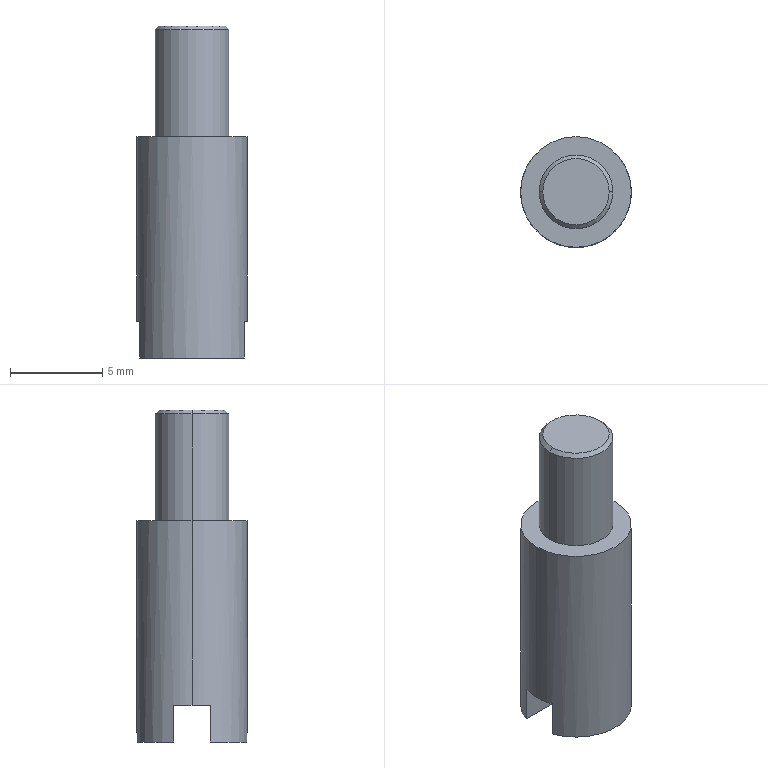Part | NX | features BREP 1 | 1 solid | 13 faces | box 6 x 6 x 18 mm | volume 390.899 mm3 | plane 7 | cylinder 4 | cone 2 | commonest cylinder face diameters 4 x2 6 x2
STEP:
#1=CARTESIAN_POINT('',(-2.828,1.,2.));
#2=VERTEX_POINT('',#1);
#3=CARTESIAN_POINT('',(2.828,1.,2.));
#4=VERTEX_POINT('',#3);
#5=CARTESIAN_POINT('',(3.,1.,2.));
#6=DIRECTION('',(1.,0.,0.));
#7=VECTOR('',#6,1000.);
#8=LINE('',#5,#7);
#9=EDGE_CURVE('',#2,#4,#8,.T.);
#10=ORIENTED_EDGE('',*,*,#9,.F.);
#11=CARTESIAN_POINT('',(-2.828,1.,0.));
#12=VERTEX_POINT('',#11);
#13=CARTESIAN_POINT('',(-2.828,1.,12.));
#14=DIRECTION('',(0.,0.,1.));
#15=VECTOR('',#14,1000.);
#16=LINE('',#13,#15);
#17=EDGE_CURVE('',#12,#2,#16,.T.);
#18=ORIENTED_EDGE('',*,*,#17,.F.);
#19=CARTESIAN_POINT('',(2.828,1.,0.));
#20=VERTEX_POINT('',#19);
#21=CARTESIAN_POINT('',(0.,1.,0.));
#22=DIRECTION('',(-1.,0.,0.));
#23=VECTOR('',#22,1000.);
#24=LINE('',#21,#23);
#25=EDGE_CURVE('',#20,#12,#24,.T.);
#26=ORIENTED_EDGE('',*,*,#25,.F.);
#27=CARTESIAN_POINT('',(2.828,1.,12.));
#28=DIRECTION('',(0.,0.,-1.));
#29=VECTOR('',#28,1000.);
#30=LINE('',#27,#29);
#31=EDGE_CURVE('',#4,#20,#30,.T.);
#32=ORIENTED_EDGE('',*,*,#31,.F.);
#33=EDGE_LOOP('',(#10,#18,#26,#32));
#34=FACE_BOUND('',#33,.T.);
#35=CARTESIAN_POINT('',(3.,1.,2.));
#36=DIRECTION('',(0.,1.,0.));
#37=DIRECTION('',(0.,0.,1.));
#38=AXIS2_PLACEMENT_3D('',#35,#36,#37);
#39=PLANE('',#38);
#40=ADVANCED_FACE('',(#34),#39,.F.);
#41=CARTESIAN_POINT('',(2.828,-1.,2.));
#42=VERTEX_POINT('',#41);
#43=CARTESIAN_POINT('',(-2.828,-1.,2.));
#44=VERTEX_POINT('',#43);
#45=CARTESIAN_POINT('',(3.,-1.,2.));
#46=DIRECTION('',(-1.,0.,0.));
#47=VECTOR('',#46,1000.);
#48=LINE('',#45,#47);
#49=EDGE_CURVE('',#42,#44,#48,.T.);
#50=ORIENTED_EDGE('',*,*,#49,.F.);
#51=CARTESIAN_POINT('',(2.828,-1.,0.));
#52=VERTEX_POINT('',#51);
#53=CARTESIAN_POINT('',(2.828,-1.,12.));
#54=DIRECTION('',(0.,0.,1.));
#55=VECTOR('',#54,1000.);
#56=LINE('',#53,#55);
#57=EDGE_CURVE('',#52,#42,#56,.T.);
#58=ORIENTED_EDGE('',*,*,#57,.F.);
#59=CARTESIAN_POINT('',(-2.828,-1.,0.));
#60=VERTEX_POINT('',#59);
#61=CARTESIAN_POINT('',(0.,-1.,0.));
#62=DIRECTION('',(1.,0.,0.));
#63=VECTOR('',#62,1000.);
#64=LINE('',#61,#63);
#65=EDGE_CURVE('',#60,#52,#64,.T.);
#66=ORIENTED_EDGE('',*,*,#65,.F.);
#67=CARTESIAN_POINT('',(-2.828,-1.,12.));
#68=DIRECTION('',(0.,0.,-1.));
#69=VECTOR('',#68,1000.);
#70=LINE('',#67,#69);
#71=EDGE_CURVE('',#44,#60,#70,.T.);
#72=ORIENTED_EDGE('',*,*,#71,.F.);
#73=EDGE_LOOP('',(#50,#58,#66,#72));
#74=FACE_BOUND('',#73,.T.);
#75=CARTESIAN_POINT('',(3.,-1.,2.));
#76=DIRECTION('',(0.,-1.,0.));
#77=DIRECTION('',(0.,0.,-1.));
#78=AXIS2_PLACEMENT_3D('',#75,#76,#77);
#79=PLANE('',#78);
#80=ADVANCED_FACE('',(#74),#79,.F.);
#81=ORIENTED_EDGE('',*,*,#9,.T.);
#82=CARTESIAN_POINT('',(3.,0.,2.));
#83=VERTEX_POINT('',#82);
#84=CARTESIAN_POINT('',(0.,0.,2.));
#85=DIRECTION('',(0.,0.,1.));
#86=DIRECTION('',(1.,0.,0.));
#87=AXIS2_PLACEMENT_3D('',#84,#85,#86);
#88=CIRCLE('',#87,3.);
#89=EDGE_CURVE('',#83,#4,#88,.T.);
#90=ORIENTED_EDGE('',*,*,#89,.F.);
#91=CARTESIAN_POINT('',(0.,0.,2.));
#92=DIRECTION('',(0.,0.,1.));
#93=DIRECTION('',(1.,0.,0.));
#94=AXIS2_PLACEMENT_3D('',#91,#92,#93);
#95=CIRCLE('',#94,3.);
#96=EDGE_CURVE('',#42,#83,#95,.T.);
#97=ORIENTED_EDGE('',*,*,#96,.F.);
#98=ORIENTED_EDGE('',*,*,#49,.T.);
#99=CARTESIAN_POINT('',(-3.,0.,2.));
#100=VERTEX_POINT('',#99);
#101=CARTESIAN_POINT('',(0.,0.,2.));
#102=DIRECTION('',(0.,0.,1.));
#103=DIRECTION('',(1.,0.,0.));
#104=AXIS2_PLACEMENT_3D('',#101,#102,#103);
#105=CIRCLE('',#104,3.);
#106=EDGE_CURVE('',#100,#44,#105,.T.);
#107=ORIENTED_EDGE('',*,*,#106,.F.);
#108=CARTESIAN_POINT('',(0.,0.,2.));
#109=DIRECTION('',(0.,0.,1.));
#110=DIRECTION('',(1.,0.,0.));
#111=AXIS2_PLACEMENT_3D('',#108,#109,#110);
#112=CIRCLE('',#111,3.);
#113=EDGE_CURVE('',#2,#100,#112,.T.);
#114=ORIENTED_EDGE('',*,*,#113,.F.);
#115=EDGE_LOOP('',(#81,#90,#97,#98,#107,#114));
#116=FACE_BOUND('',#115,.T.);
#117=CARTESIAN_POINT('',(0.,0.,2.));
#118=DIRECTION('',(0.,0.,1.));
#119=DIRECTION('',(1.,0.,0.));
#120=AXIS2_PLACEMENT_3D('',#117,#118,#119);
#121=PLANE('',#120);
#122=ADVANCED_FACE('',(#116),#121,.F.);
#123=CARTESIAN_POINT('',(1.8,0.,18.));
#124=VERTEX_POINT('',#123);
#125=CARTESIAN_POINT('',(2.,0.,17.8));
#126=VERTEX_POINT('',#125);
#127=CARTESIAN_POINT('',(1.8,0.,18.));
#128=DIRECTION('',(0.7071,0.,-0.7071));
#129=VECTOR('',#128,1000.);
#130=LINE('',#127,#129);
#131=EDGE_CURVE('',#124,#126,#130,.T.);
#132=ORIENTED_EDGE('',*,*,#131,.F.);
#133=CARTESIAN_POINT('',(-1.8,0.,18.));
#134=VERTEX_POINT('',#133);
#135=CARTESIAN_POINT('',(0.,0.,18.));
#136=DIRECTION('',(0.,0.,1.));
#137=DIRECTION('',(1.,0.,0.));
#138=AXIS2_PLACEMENT_3D('',#135,#136,#137);
#139=CIRCLE('',#138,1.8);
#140=EDGE_CURVE('',#134,#124,#139,.T.);
#141=ORIENTED_EDGE('',*,*,#140,.F.);
#142=CARTESIAN_POINT('',(-2.,0.,17.8));
#143=VERTEX_POINT('',#142);
#144=CARTESIAN_POINT('',(-1.8,0.,18.));
#145=DIRECTION('',(-0.7071,0.,-0.7071));
#146=VECTOR('',#145,1000.);
#147=LINE('',#144,#146);
#148=EDGE_CURVE('',#134,#143,#147,.T.);
#149=ORIENTED_EDGE('',*,*,#148,.T.);
#150=CARTESIAN_POINT('',(0.,0.,17.8));
#151=DIRECTION('',(0.,0.,-1.));
#152=DIRECTION('',(1.,0.,0.));
#153=AXIS2_PLACEMENT_3D('',#150,#151,#152);
#154=CIRCLE('',#153,2.);
#155=EDGE_CURVE('',#126,#143,#154,.T.);
#156=ORIENTED_EDGE('',*,*,#155,.F.);
#157=EDGE_LOOP('',(#132,#141,#149,#156));
#158=FACE_BOUND('',#157,.T.);
#159=CARTESIAN_POINT('',(0.,0.,18.));
#160=DIRECTION('',(0.,0.,-1.));
#161=DIRECTION('',(-1.,0.,0.));
#162=AXIS2_PLACEMENT_3D('',#159,#160,#161);
#163=CONICAL_SURFACE('',#162,1.8,0.7854);
#164=ADVANCED_FACE('',(#158),#163,.T.);
#165=ORIENTED_EDGE('',*,*,#140,.T.);
#166=CARTESIAN_POINT('',(0.,0.,18.));
#167=DIRECTION('',(0.,0.,1.));
#168=DIRECTION('',(1.,0.,0.));
#169=AXIS2_PLACEMENT_3D('',#166,#167,#168);
#170=CIRCLE('',#169,1.8);
#171=EDGE_CURVE('',#124,#134,#170,.T.);
#172=ORIENTED_EDGE('',*,*,#171,.T.);
#173=EDGE_LOOP('',(#165,#172));
#174=FACE_BOUND('',#173,.T.);
#175=CARTESIAN_POINT('',(0.,0.,18.));
#176=DIRECTION('',(0.,0.,1.));
#177=DIRECTION('',(1.,0.,0.));
#178=AXIS2_PLACEMENT_3D('',#175,#176,#177);
#179=PLANE('',#178);
#180=ADVANCED_FACE('',(#174),#179,.T.);
#181=CARTESIAN_POINT('',(2.,0.,12.));
#182=VERTEX_POINT('',#181);
#183=CARTESIAN_POINT('',(2.,0.,18.));
#184=DIRECTION('',(0.,0.,-1.));
#185=VECTOR('',#184,1000.);
#186=LINE('',#183,#185);
#187=EDGE_CURVE('',#126,#182,#186,.T.);
#188=ORIENTED_EDGE('',*,*,#187,.F.);
#189=ORIENTED_EDGE('',*,*,#155,.T.);
#190=CARTESIAN_POINT('',(-2.,0.,12.));
#191=VERTEX_POINT('',#190);
#192=CARTESIAN_POINT('',(-2.,0.,18.));
#193=DIRECTION('',(0.,0.,-1.));
#194=VECTOR('',#193,1000.);
#195=LINE('',#192,#194);
#196=EDGE_CURVE('',#143,#191,#195,.T.);
#197=ORIENTED_EDGE('',*,*,#196,.T.);
#198=CARTESIAN_POINT('',(0.,0.,12.));
#199=DIRECTION('',(0.,0.,1.));
#200=DIRECTION('',(1.,0.,0.));
#201=AXIS2_PLACEMENT_3D('',#198,#199,#200);
#202=CIRCLE('',#201,2.);
#203=EDGE_CURVE('',#191,#182,#202,.T.);
#204=ORIENTED_EDGE('',*,*,#203,.T.);
#205=EDGE_LOOP('',(#188,#189,#197,#204));
#206=FACE_BOUND('',#205,.T.);
#207=CARTESIAN_POINT('',(0.,0.,18.));
#208=DIRECTION('',(0.,0.,-1.));
#209=DIRECTION('',(-1.,0.,0.));
#210=AXIS2_PLACEMENT_3D('',#207,#208,#209);
#211=CYLINDRICAL_SURFACE('',#210,2.);
#212=ADVANCED_FACE('',(#206),#211,.T.);
#213=CARTESIAN_POINT('',(0.,0.,0.));
#214=DIRECTION('',(0.,0.,1.));
#215=DIRECTION('',(1.,0.,0.));
#216=AXIS2_PLACEMENT_3D('',#213,#214,#215);
#217=CIRCLE('',#216,3.);
#218=EDGE_CURVE('',#20,#12,#217,.T.);
#219=ORIENTED_EDGE('',*,*,#218,.F.);
#220=ORIENTED_EDGE('',*,*,#25,.T.);
#221=EDGE_LOOP('',(#219,#220));
#222=FACE_BOUND('',#221,.T.);
#223=CARTESIAN_POINT('',(0.,0.,0.));
#224=DIRECTION('',(0.,0.,1.));
#225=DIRECTION('',(1.,0.,0.));
#226=AXIS2_PLACEMENT_3D('',#223,#224,#225);
#227=PLANE('',#226);
#228=ADVANCED_FACE('',(#222),#227,.F.);
#229=CARTESIAN_POINT('',(-3.,0.,12.));
#230=VERTEX_POINT('',#229);
#231=CARTESIAN_POINT('',(3.,0.,12.));
#232=VERTEX_POINT('',#231);
#233=CARTESIAN_POINT('',(0.,0.,12.));
#234=DIRECTION('',(0.,0.,1.));
#235=DIRECTION('',(1.,0.,0.));
#236=AXIS2_PLACEMENT_3D('',#233,#234,#235);
#237=CIRCLE('',#236,3.);
#238=EDGE_CURVE('',#230,#232,#237,.T.);
#239=ORIENTED_EDGE('',*,*,#238,.T.);
#240=CARTESIAN_POINT('',(0.,0.,12.));
#241=DIRECTION('',(0.,0.,1.));
#242=DIRECTION('',(1.,0.,0.));
#243=AXIS2_PLACEMENT_3D('',#240,#241,#242);
#244=CIRCLE('',#243,3.);
#245=EDGE_CURVE('',#232,#230,#244,.T.);
#246=ORIENTED_EDGE('',*,*,#245,.T.);
#247=EDGE_LOOP('',(#239,#246));
#248=FACE_BOUND('',#247,.T.);
#249=ORIENTED_EDGE('',*,*,#203,.F.);
#250=CARTESIAN_POINT('',(0.,0.,12.));
#251=DIRECTION('',(0.,0.,1.));
#252=DIRECTION('',(1.,0.,0.));
#253=AXIS2_PLACEMENT_3D('',#250,#251,#252);
#254=CIRCLE('',#253,2.);
#255=EDGE_CURVE('',#182,#191,#254,.T.);
#256=ORIENTED_EDGE('',*,*,#255,.F.);
#257=EDGE_LOOP('',(#249,#256));
#258=FACE_BOUND('',#257,.T.);
#259=CARTESIAN_POINT('',(0.,0.,12.));
#260=DIRECTION('',(0.,0.,1.));
#261=DIRECTION('',(1.,0.,0.));
#262=AXIS2_PLACEMENT_3D('',#259,#260,#261);
#263=PLANE('',#262);
#264=ADVANCED_FACE('',(#248,#258),#263,.T.);
#265=CARTESIAN_POINT('',(3.,0.,12.));
#266=DIRECTION('',(0.,0.,-1.));
#267=VECTOR('',#266,1000.);
#268=LINE('',#265,#267);
#269=EDGE_CURVE('',#232,#83,#268,.T.);
#270=ORIENTED_EDGE('',*,*,#269,.F.);
#271=ORIENTED_EDGE('',*,*,#238,.F.);
#272=CARTESIAN_POINT('',(-3.,0.,12.));
#273=DIRECTION('',(0.,0.,-1.));
#274=VECTOR('',#273,1000.);
#275=LINE('',#272,#274);
#276=EDGE_CURVE('',#230,#100,#275,.T.);
#277=ORIENTED_EDGE('',*,*,#276,.T.);
#278=ORIENTED_EDGE('',*,*,#106,.T.);
#279=ORIENTED_EDGE('',*,*,#71,.T.);
#280=CARTESIAN_POINT('',(0.,0.,0.));
#281=DIRECTION('',(0.,0.,1.));
#282=DIRECTION('',(1.,0.,0.));
#283=AXIS2_PLACEMENT_3D('',#280,#281,#282);
#284=CIRCLE('',#283,3.);
#285=EDGE_CURVE('',#60,#52,#284,.T.);
#286=ORIENTED_EDGE('',*,*,#285,.T.);
#287=ORIENTED_EDGE('',*,*,#57,.T.);
#288=ORIENTED_EDGE('',*,*,#96,.T.);
#289=EDGE_LOOP('',(#270,#271,#277,#278,#279,#286,#287,#288));
#290=FACE_BOUND('',#289,.T.);
#291=CARTESIAN_POINT('',(0.,0.,12.));
#292=DIRECTION('',(0.,0.,-1.));
#293=DIRECTION('',(-1.,0.,0.));
#294=AXIS2_PLACEMENT_3D('',#291,#292,#293);
#295=CYLINDRICAL_SURFACE('',#294,3.);
#296=ADVANCED_FACE('',(#290),#295,.T.);
#297=ORIENTED_EDGE('',*,*,#285,.F.);
#298=ORIENTED_EDGE('',*,*,#65,.T.);
#299=EDGE_LOOP('',(#297,#298));
#300=FACE_BOUND('',#299,.T.);
#301=CARTESIAN_POINT('',(0.,0.,0.));
#302=DIRECTION('',(0.,0.,1.));
#303=DIRECTION('',(1.,0.,0.));
#304=AXIS2_PLACEMENT_3D('',#301,#302,#303);
#305=PLANE('',#304);
#306=ADVANCED_FACE('',(#300),#305,.F.);
#307=ORIENTED_EDGE('',*,*,#245,.F.);
#308=ORIENTED_EDGE('',*,*,#269,.T.);
#309=ORIENTED_EDGE('',*,*,#89,.T.);
#310=ORIENTED_EDGE('',*,*,#31,.T.);
#311=ORIENTED_EDGE('',*,*,#218,.T.);
#312=ORIENTED_EDGE('',*,*,#17,.T.);
#313=ORIENTED_EDGE('',*,*,#113,.T.);
#314=ORIENTED_EDGE('',*,*,#276,.F.);
#315=EDGE_LOOP('',(#307,#308,#309,#310,#311,#312,#313,#314));
#316=FACE_BOUND('',#315,.T.);
#317=CARTESIAN_POINT('',(0.,0.,12.));
#318=DIRECTION('',(0.,0.,-1.));
#319=DIRECTION('',(-1.,0.,0.));
#320=AXIS2_PLACEMENT_3D('',#317,#318,#319);
#321=CYLINDRICAL_SURFACE('',#320,3.);
#322=ADVANCED_FACE('',(#316),#321,.T.);
#323=CARTESIAN_POINT('',(0.,0.,17.8));
#324=DIRECTION('',(0.,0.,-1.));
#325=DIRECTION('',(1.,0.,0.));
#326=AXIS2_PLACEMENT_3D('',#323,#324,#325);
#327=CIRCLE('',#326,2.);
#328=EDGE_CURVE('',#143,#126,#327,.T.);
#329=ORIENTED_EDGE('',*,*,#328,.T.);
#330=ORIENTED_EDGE('',*,*,#187,.T.);
#331=ORIENTED_EDGE('',*,*,#255,.T.);
#332=ORIENTED_EDGE('',*,*,#196,.F.);
#333=EDGE_LOOP('',(#329,#330,#331,#332));
#334=FACE_BOUND('',#333,.T.);
#335=CARTESIAN_POINT('',(0.,0.,18.));
#336=DIRECTION('',(0.,0.,-1.));
#337=DIRECTION('',(-1.,0.,0.));
#338=AXIS2_PLACEMENT_3D('',#335,#336,#337);
#339=CYLINDRICAL_SURFACE('',#338,2.);
#340=ADVANCED_FACE('',(#334),#339,.T.);
#341=ORIENTED_EDGE('',*,*,#171,.F.);
#342=ORIENTED_EDGE('',*,*,#131,.T.);
#343=ORIENTED_EDGE('',*,*,#328,.F.);
#344=ORIENTED_EDGE('',*,*,#148,.F.);
#345=EDGE_LOOP('',(#341,#342,#343,#344));
#346=FACE_BOUND('',#345,.T.);
#347=CARTESIAN_POINT('',(0.,0.,18.));
#348=DIRECTION('',(0.,0.,-1.));
#349=DIRECTION('',(-1.,0.,0.));
#350=AXIS2_PLACEMENT_3D('',#347,#348,#349);
#351=CONICAL_SURFACE('',#350,1.8,0.7854);
#352=ADVANCED_FACE('',(#346),#351,.T.);
#353=CLOSED_SHELL('',(#40,#80,#122,#164,#180,#212,#228,#264,#296,#306,#322,#340,#352));
#354=MANIFOLD_SOLID_BREP('',#353);
#355=(LENGTH_UNIT()NAMED_UNIT(*)SI_UNIT(.MILLI.,.METRE.));
#356=UNCERTAINTY_MEASURE_WITH_UNIT(LENGTH_MEASURE(0.00001),#355,'','');
#357=(NAMED_UNIT(*)PLANE_ANGLE_UNIT()SI_UNIT($,.RADIAN.));
#358=(NAMED_UNIT(*)SI_UNIT($,.STERADIAN.)SOLID_ANGLE_UNIT());
#359=(GEOMETRIC_REPRESENTATION_CONTEXT(3)GLOBAL_UNCERTAINTY_ASSIGNED_CONTEXT((#356))GLOBAL_UNIT_ASSIGNED_CONTEXT((#355,#357,#358))REPRESENTATION_CONTEXT('',''));
#360=ADVANCED_BREP_SHAPE_REPRESENTATION('',(#354),#359);